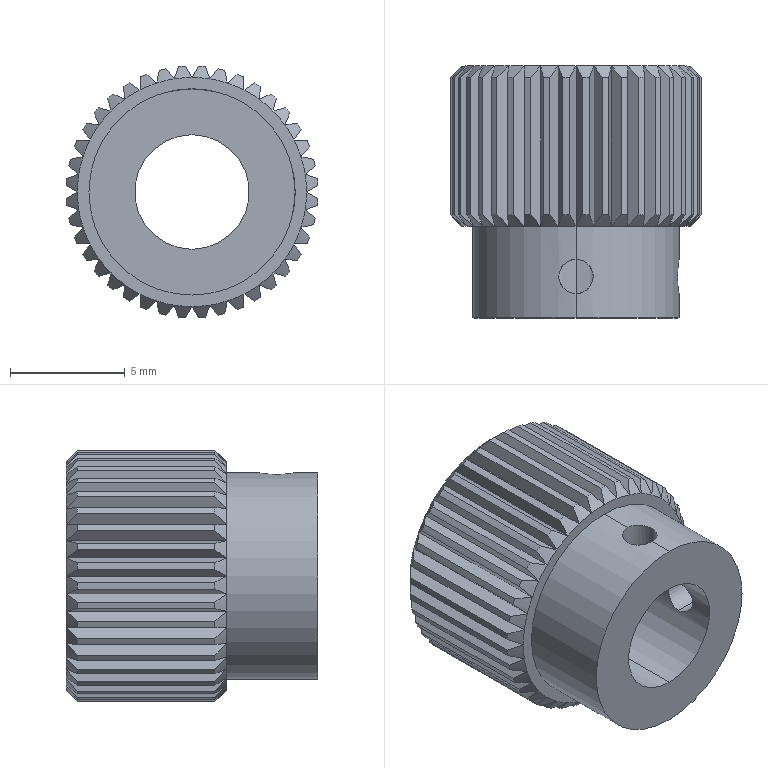Part | SolidWorks | features ICE 3, CirPattern 1, Revolution 1 | 1 solid | 211 faces | box 10.985 x 11 x 10.985 mm | volume 652.018 mm3 | plane 83 | cone 80 | cylinder 48 | commonest cylinder face diameters 11 x40 1.5 x4 5 x2 9 x2